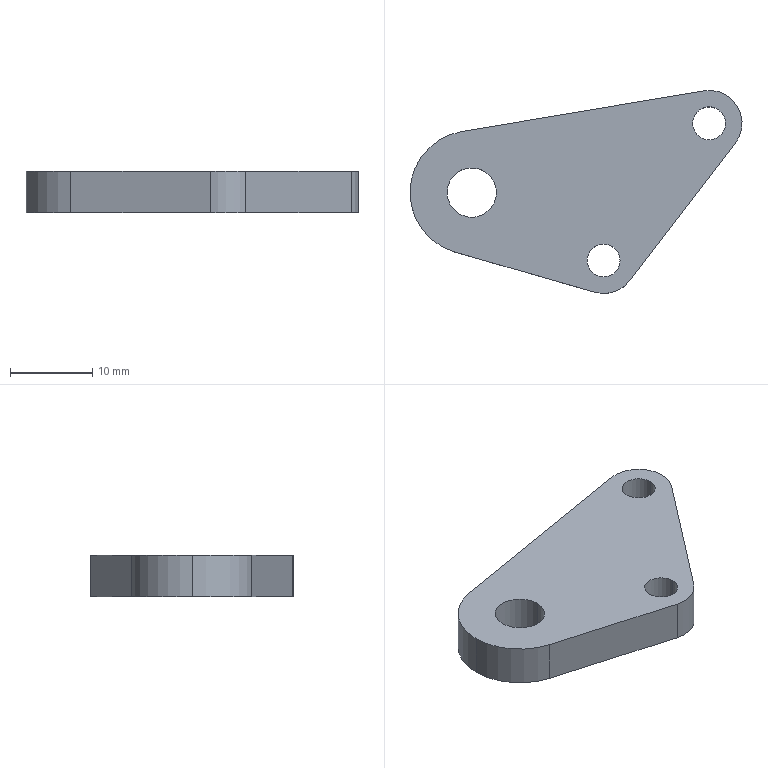Part | SolidWorks | features Extrusion 1 | 1 solid | 15 faces | box 40.3 x 24.65 x 5 mm | volume 2970 mm3 | cylinder 10 | plane 5 | commonest cylinder face diameters 4 x4 6 x2 8 x2 15 x2
STEP:
#1=CARTESIAN_POINT('',(10.8,16.65,5.));
#2=VERTEX_POINT('',#1);
#3=CARTESIAN_POINT('',(14.8,16.65,5.));
#4=VERTEX_POINT('',#3);
#5=CARTESIAN_POINT('',(12.8,16.65,5.));
#6=DIRECTION('',(0.,0.,1.));
#7=DIRECTION('',(1.,0.,0.));
#8=AXIS2_PLACEMENT_3D('',#5,#6,#7);
#9=CIRCLE('',#8,2.);
#10=EDGE_CURVE('',#2,#4,#9,.T.);
#11=ORIENTED_EDGE('',*,*,#10,.T.);
#12=CARTESIAN_POINT('',(14.8,16.65,0.));
#13=VERTEX_POINT('',#12);
#14=CARTESIAN_POINT('',(14.8,16.65,5.));
#15=DIRECTION('',(0.,0.,-1.));
#16=VECTOR('',#15,1000.);
#17=LINE('',#14,#16);
#18=EDGE_CURVE('',#4,#13,#17,.T.);
#19=ORIENTED_EDGE('',*,*,#18,.T.);
#20=CARTESIAN_POINT('',(10.8,16.65,0.));
#21=VERTEX_POINT('',#20);
#22=CARTESIAN_POINT('',(12.8,16.65,0.));
#23=DIRECTION('',(0.,0.,1.));
#24=DIRECTION('',(1.,0.,0.));
#25=AXIS2_PLACEMENT_3D('',#22,#23,#24);
#26=CIRCLE('',#25,2.);
#27=EDGE_CURVE('',#21,#13,#26,.T.);
#28=ORIENTED_EDGE('',*,*,#27,.F.);
#29=CARTESIAN_POINT('',(10.8,16.65,5.));
#30=DIRECTION('',(0.,0.,-1.));
#31=VECTOR('',#30,1000.);
#32=LINE('',#29,#31);
#33=EDGE_CURVE('',#2,#21,#32,.T.);
#34=ORIENTED_EDGE('',*,*,#33,.F.);
#35=EDGE_LOOP('',(#11,#19,#28,#34));
#36=FACE_OUTER_BOUND('',#35,.T.);
#37=CARTESIAN_POINT('',(12.8,16.65,5.));
#38=DIRECTION('',(0.,0.,-1.));
#39=DIRECTION('',(-1.,0.,0.));
#40=AXIS2_PLACEMENT_3D('',#37,#38,#39);
#41=CYLINDRICAL_SURFACE('',#40,2.);
#42=ADVANCED_FACE('',(#36),#41,.F.);
#43=CARTESIAN_POINT('',(-19.,8.25,5.));
#44=VERTEX_POINT('',#43);
#45=CARTESIAN_POINT('',(-13.,8.25,5.));
#46=VERTEX_POINT('',#45);
#47=CARTESIAN_POINT('',(-16.,8.25,5.));
#48=DIRECTION('',(0.,0.,1.));
#49=DIRECTION('',(1.,0.,0.));
#50=AXIS2_PLACEMENT_3D('',#47,#48,#49);
#51=CIRCLE('',#50,3.);
#52=EDGE_CURVE('',#44,#46,#51,.T.);
#53=ORIENTED_EDGE('',*,*,#52,.T.);
#54=CARTESIAN_POINT('',(-13.,8.25,0.));
#55=VERTEX_POINT('',#54);
#56=CARTESIAN_POINT('',(-13.,8.25,5.));
#57=DIRECTION('',(0.,0.,-1.));
#58=VECTOR('',#57,1000.);
#59=LINE('',#56,#58);
#60=EDGE_CURVE('',#46,#55,#59,.T.);
#61=ORIENTED_EDGE('',*,*,#60,.T.);
#62=CARTESIAN_POINT('',(-19.,8.25,0.));
#63=VERTEX_POINT('',#62);
#64=CARTESIAN_POINT('',(-16.,8.25,0.));
#65=DIRECTION('',(0.,0.,1.));
#66=DIRECTION('',(1.,0.,0.));
#67=AXIS2_PLACEMENT_3D('',#64,#65,#66);
#68=CIRCLE('',#67,3.);
#69=EDGE_CURVE('',#63,#55,#68,.T.);
#70=ORIENTED_EDGE('',*,*,#69,.F.);
#71=CARTESIAN_POINT('',(-19.,8.25,5.));
#72=DIRECTION('',(0.,0.,-1.));
#73=VECTOR('',#72,1000.);
#74=LINE('',#71,#73);
#75=EDGE_CURVE('',#44,#63,#74,.T.);
#76=ORIENTED_EDGE('',*,*,#75,.F.);
#77=EDGE_LOOP('',(#53,#61,#70,#76));
#78=FACE_OUTER_BOUND('',#77,.T.);
#79=CARTESIAN_POINT('',(-16.,8.25,5.));
#80=DIRECTION('',(0.,0.,-1.));
#81=DIRECTION('',(-1.,0.,0.));
#82=AXIS2_PLACEMENT_3D('',#79,#80,#81);
#83=CYLINDRICAL_SURFACE('',#82,3.);
#84=ADVANCED_FACE('',(#78),#83,.F.);
#85=CARTESIAN_POINT('',(-2.,0.,5.));
#86=VERTEX_POINT('',#85);
#87=CARTESIAN_POINT('',(2.,0.,5.));
#88=VERTEX_POINT('',#87);
#89=CARTESIAN_POINT('',(0.,0.,5.));
#90=DIRECTION('',(0.,0.,1.));
#91=DIRECTION('',(1.,0.,0.));
#92=AXIS2_PLACEMENT_3D('',#89,#90,#91);
#93=CIRCLE('',#92,2.);
#94=EDGE_CURVE('',#86,#88,#93,.T.);
#95=ORIENTED_EDGE('',*,*,#94,.T.);
#96=CARTESIAN_POINT('',(2.,0.,0.));
#97=VERTEX_POINT('',#96);
#98=CARTESIAN_POINT('',(2.,0.,5.));
#99=DIRECTION('',(0.,0.,-1.));
#100=VECTOR('',#99,1000.);
#101=LINE('',#98,#100);
#102=EDGE_CURVE('',#88,#97,#101,.T.);
#103=ORIENTED_EDGE('',*,*,#102,.T.);
#104=CARTESIAN_POINT('',(-2.,0.,0.));
#105=VERTEX_POINT('',#104);
#106=CARTESIAN_POINT('',(0.,0.,0.));
#107=DIRECTION('',(0.,0.,1.));
#108=DIRECTION('',(1.,0.,0.));
#109=AXIS2_PLACEMENT_3D('',#106,#107,#108);
#110=CIRCLE('',#109,2.);
#111=EDGE_CURVE('',#105,#97,#110,.T.);
#112=ORIENTED_EDGE('',*,*,#111,.F.);
#113=CARTESIAN_POINT('',(-2.,0.,5.));
#114=DIRECTION('',(0.,0.,-1.));
#115=VECTOR('',#114,1000.);
#116=LINE('',#113,#115);
#117=EDGE_CURVE('',#86,#105,#116,.T.);
#118=ORIENTED_EDGE('',*,*,#117,.F.);
#119=EDGE_LOOP('',(#95,#103,#112,#118));
#120=FACE_OUTER_BOUND('',#119,.T.);
#121=CARTESIAN_POINT('',(0.,0.,5.));
#122=DIRECTION('',(0.,0.,-1.));
#123=DIRECTION('',(-1.,0.,0.));
#124=AXIS2_PLACEMENT_3D('',#121,#122,#123);
#125=CYLINDRICAL_SURFACE('',#124,2.);
#126=ADVANCED_FACE('',(#120),#125,.F.);
#127=CARTESIAN_POINT('',(-23.5,8.25,5.));
#128=VERTEX_POINT('',#127);
#129=CARTESIAN_POINT('',(-18.076,1.043,5.));
#130=VERTEX_POINT('',#129);
#131=CARTESIAN_POINT('',(-16.,8.25,5.));
#132=DIRECTION('',(0.,0.,1.));
#133=DIRECTION('',(1.,0.,0.));
#134=AXIS2_PLACEMENT_3D('',#131,#132,#133);
#135=CIRCLE('',#134,7.5);
#136=EDGE_CURVE('',#128,#130,#135,.T.);
#137=ORIENTED_EDGE('',*,*,#136,.F.);
#138=CARTESIAN_POINT('',(-23.5,8.25,0.));
#139=VERTEX_POINT('',#138);
#140=CARTESIAN_POINT('',(-23.5,8.25,5.));
#141=DIRECTION('',(0.,0.,-1.));
#142=VECTOR('',#141,1000.);
#143=LINE('',#140,#142);
#144=EDGE_CURVE('',#128,#139,#143,.T.);
#145=ORIENTED_EDGE('',*,*,#144,.T.);
#146=CARTESIAN_POINT('',(-18.076,1.043,0.));
#147=VERTEX_POINT('',#146);
#148=CARTESIAN_POINT('',(-16.,8.25,0.));
#149=DIRECTION('',(0.,0.,1.));
#150=DIRECTION('',(1.,0.,0.));
#151=AXIS2_PLACEMENT_3D('',#148,#149,#150);
#152=CIRCLE('',#151,7.5);
#153=EDGE_CURVE('',#139,#147,#152,.T.);
#154=ORIENTED_EDGE('',*,*,#153,.T.);
#155=CARTESIAN_POINT('',(-18.076,1.043,5.));
#156=DIRECTION('',(0.,0.,-1.));
#157=VECTOR('',#156,1000.);
#158=LINE('',#155,#157);
#159=EDGE_CURVE('',#130,#147,#158,.T.);
#160=ORIENTED_EDGE('',*,*,#159,.F.);
#161=EDGE_LOOP('',(#137,#145,#154,#160));
#162=FACE_OUTER_BOUND('',#161,.T.);
#163=CARTESIAN_POINT('',(-16.,8.25,5.));
#164=DIRECTION('',(0.,0.,-1.));
#165=DIRECTION('',(-1.,0.,0.));
#166=AXIS2_PLACEMENT_3D('',#163,#164,#165);
#167=CYLINDRICAL_SURFACE('',#166,7.5);
#168=ADVANCED_FACE('',(#162),#167,.T.);
#169=ORIENTED_EDGE('',*,*,#52,.F.);
#170=CARTESIAN_POINT('',(-16.,8.25,5.));
#171=DIRECTION('',(0.,0.,1.));
#172=DIRECTION('',(1.,0.,0.));
#173=AXIS2_PLACEMENT_3D('',#170,#171,#172);
#174=CIRCLE('',#173,3.);
#175=EDGE_CURVE('',#46,#44,#174,.T.);
#176=ORIENTED_EDGE('',*,*,#175,.F.);
#177=EDGE_LOOP('',(#169,#176));
#178=FACE_BOUND('',#177,.T.);
#179=CARTESIAN_POINT('',(-17.246,15.646,5.));
#180=VERTEX_POINT('',#179);
#181=CARTESIAN_POINT('',(-16.,8.25,5.));
#182=DIRECTION('',(0.,0.,1.));
#183=DIRECTION('',(1.,0.,0.));
#184=AXIS2_PLACEMENT_3D('',#181,#182,#183);
#185=CIRCLE('',#184,7.5);
#186=EDGE_CURVE('',#180,#128,#185,.T.);
#187=ORIENTED_EDGE('',*,*,#186,.T.);
#188=ORIENTED_EDGE('',*,*,#136,.T.);
#189=CARTESIAN_POINT('',(-1.107,-3.844,5.));
#190=VERTEX_POINT('',#189);
#191=CARTESIAN_POINT('',(-18.076,1.043,5.));
#192=DIRECTION('',(0.9609,-0.2767,0.));
#193=VECTOR('',#192,1000.);
#194=LINE('',#191,#193);
#195=EDGE_CURVE('',#130,#190,#194,.T.);
#196=ORIENTED_EDGE('',*,*,#195,.T.);
#197=CARTESIAN_POINT('',(3.171,-2.438,5.));
#198=VERTEX_POINT('',#197);
#199=CARTESIAN_POINT('',(0.,0.,5.));
#200=DIRECTION('',(0.,0.,1.));
#201=DIRECTION('',(1.,0.,0.));
#202=AXIS2_PLACEMENT_3D('',#199,#200,#201);
#203=CIRCLE('',#202,4.);
#204=EDGE_CURVE('',#190,#198,#203,.T.);
#205=ORIENTED_EDGE('',*,*,#204,.T.);
#206=CARTESIAN_POINT('',(15.971,14.212,5.));
#207=VERTEX_POINT('',#206);
#208=CARTESIAN_POINT('',(15.971,14.212,5.));
#209=DIRECTION('',(0.6095,0.7928,0.));
#210=VECTOR('',#209,1000.);
#211=LINE('',#208,#210);
#212=EDGE_CURVE('',#198,#207,#211,.T.);
#213=ORIENTED_EDGE('',*,*,#212,.T.);
#214=CARTESIAN_POINT('',(12.136,20.594,5.));
#215=VERTEX_POINT('',#214);
#216=CARTESIAN_POINT('',(12.8,16.65,5.));
#217=DIRECTION('',(0.,0.,1.));
#218=DIRECTION('',(1.,0.,0.));
#219=AXIS2_PLACEMENT_3D('',#216,#217,#218);
#220=CIRCLE('',#219,4.);
#221=EDGE_CURVE('',#207,#215,#220,.T.);
#222=ORIENTED_EDGE('',*,*,#221,.T.);
#223=CARTESIAN_POINT('',(-17.246,15.646,5.));
#224=DIRECTION('',(-0.9861,-0.1661,0.));
#225=VECTOR('',#224,1000.);
#226=LINE('',#223,#225);
#227=EDGE_CURVE('',#215,#180,#226,.T.);
#228=ORIENTED_EDGE('',*,*,#227,.T.);
#229=EDGE_LOOP('',(#187,#188,#196,#205,#213,#222,#228));
#230=FACE_OUTER_BOUND('',#229,.T.);
#231=ORIENTED_EDGE('',*,*,#94,.F.);
#232=CARTESIAN_POINT('',(0.,0.,5.));
#233=DIRECTION('',(0.,0.,1.));
#234=DIRECTION('',(1.,0.,0.));
#235=AXIS2_PLACEMENT_3D('',#232,#233,#234);
#236=CIRCLE('',#235,2.);
#237=EDGE_CURVE('',#88,#86,#236,.T.);
#238=ORIENTED_EDGE('',*,*,#237,.F.);
#239=EDGE_LOOP('',(#231,#238));
#240=FACE_BOUND('',#239,.T.);
#241=ORIENTED_EDGE('',*,*,#10,.F.);
#242=CARTESIAN_POINT('',(12.8,16.65,5.));
#243=DIRECTION('',(0.,0.,1.));
#244=DIRECTION('',(1.,0.,0.));
#245=AXIS2_PLACEMENT_3D('',#242,#243,#244);
#246=CIRCLE('',#245,2.);
#247=EDGE_CURVE('',#4,#2,#246,.T.);
#248=ORIENTED_EDGE('',*,*,#247,.F.);
#249=EDGE_LOOP('',(#241,#248));
#250=FACE_BOUND('',#249,.T.);
#251=CARTESIAN_POINT('',(-16.,8.25,5.));
#252=DIRECTION('',(0.,0.,1.));
#253=DIRECTION('',(1.,0.,0.));
#254=AXIS2_PLACEMENT_3D('',#251,#252,#253);
#255=PLANE('',#254);
#256=ADVANCED_FACE('',(#178,#230,#240,#250),#255,.T.);
#257=CARTESIAN_POINT('',(-17.246,15.646,0.));
#258=VERTEX_POINT('',#257);
#259=CARTESIAN_POINT('',(-16.,8.25,0.));
#260=DIRECTION('',(0.,0.,1.));
#261=DIRECTION('',(1.,0.,0.));
#262=AXIS2_PLACEMENT_3D('',#259,#260,#261);
#263=CIRCLE('',#262,7.5);
#264=EDGE_CURVE('',#258,#139,#263,.T.);
#265=ORIENTED_EDGE('',*,*,#264,.F.);
#266=CARTESIAN_POINT('',(12.136,20.594,0.));
#267=VERTEX_POINT('',#266);
#268=CARTESIAN_POINT('',(-17.246,15.646,0.));
#269=DIRECTION('',(-0.9861,-0.1661,0.));
#270=VECTOR('',#269,1000.);
#271=LINE('',#268,#270);
#272=EDGE_CURVE('',#267,#258,#271,.T.);
#273=ORIENTED_EDGE('',*,*,#272,.F.);
#274=CARTESIAN_POINT('',(15.971,14.212,0.));
#275=VERTEX_POINT('',#274);
#276=CARTESIAN_POINT('',(12.8,16.65,0.));
#277=DIRECTION('',(0.,0.,1.));
#278=DIRECTION('',(1.,0.,0.));
#279=AXIS2_PLACEMENT_3D('',#276,#277,#278);
#280=CIRCLE('',#279,4.);
#281=EDGE_CURVE('',#275,#267,#280,.T.);
#282=ORIENTED_EDGE('',*,*,#281,.F.);
#283=CARTESIAN_POINT('',(3.171,-2.438,0.));
#284=VERTEX_POINT('',#283);
#285=CARTESIAN_POINT('',(15.971,14.212,0.));
#286=DIRECTION('',(0.6095,0.7928,0.));
#287=VECTOR('',#286,1000.);
#288=LINE('',#285,#287);
#289=EDGE_CURVE('',#284,#275,#288,.T.);
#290=ORIENTED_EDGE('',*,*,#289,.F.);
#291=CARTESIAN_POINT('',(-1.107,-3.844,0.));
#292=VERTEX_POINT('',#291);
#293=CARTESIAN_POINT('',(0.,0.,0.));
#294=DIRECTION('',(0.,0.,1.));
#295=DIRECTION('',(1.,0.,0.));
#296=AXIS2_PLACEMENT_3D('',#293,#294,#295);
#297=CIRCLE('',#296,4.);
#298=EDGE_CURVE('',#292,#284,#297,.T.);
#299=ORIENTED_EDGE('',*,*,#298,.F.);
#300=CARTESIAN_POINT('',(-18.076,1.043,0.));
#301=DIRECTION('',(0.9609,-0.2767,0.));
#302=VECTOR('',#301,1000.);
#303=LINE('',#300,#302);
#304=EDGE_CURVE('',#147,#292,#303,.T.);
#305=ORIENTED_EDGE('',*,*,#304,.F.);
#306=ORIENTED_EDGE('',*,*,#153,.F.);
#307=EDGE_LOOP('',(#265,#273,#282,#290,#299,#305,#306));
#308=FACE_OUTER_BOUND('',#307,.T.);
#309=ORIENTED_EDGE('',*,*,#111,.T.);
#310=CARTESIAN_POINT('',(0.,0.,0.));
#311=DIRECTION('',(0.,0.,1.));
#312=DIRECTION('',(1.,0.,0.));
#313=AXIS2_PLACEMENT_3D('',#310,#311,#312);
#314=CIRCLE('',#313,2.);
#315=EDGE_CURVE('',#97,#105,#314,.T.);
#316=ORIENTED_EDGE('',*,*,#315,.T.);
#317=EDGE_LOOP('',(#309,#316));
#318=FACE_BOUND('',#317,.T.);
#319=ORIENTED_EDGE('',*,*,#69,.T.);
#320=CARTESIAN_POINT('',(-16.,8.25,0.));
#321=DIRECTION('',(0.,0.,1.));
#322=DIRECTION('',(1.,0.,0.));
#323=AXIS2_PLACEMENT_3D('',#320,#321,#322);
#324=CIRCLE('',#323,3.);
#325=EDGE_CURVE('',#55,#63,#324,.T.);
#326=ORIENTED_EDGE('',*,*,#325,.T.);
#327=EDGE_LOOP('',(#319,#326));
#328=FACE_BOUND('',#327,.T.);
#329=ORIENTED_EDGE('',*,*,#27,.T.);
#330=CARTESIAN_POINT('',(12.8,16.65,0.));
#331=DIRECTION('',(0.,0.,1.));
#332=DIRECTION('',(1.,0.,0.));
#333=AXIS2_PLACEMENT_3D('',#330,#331,#332);
#334=CIRCLE('',#333,2.);
#335=EDGE_CURVE('',#13,#21,#334,.T.);
#336=ORIENTED_EDGE('',*,*,#335,.T.);
#337=EDGE_LOOP('',(#329,#336));
#338=FACE_BOUND('',#337,.T.);
#339=CARTESIAN_POINT('',(-16.,8.25,0.));
#340=DIRECTION('',(0.,0.,1.));
#341=DIRECTION('',(1.,0.,0.));
#342=AXIS2_PLACEMENT_3D('',#339,#340,#341);
#343=PLANE('',#342);
#344=ADVANCED_FACE('',(#308,#318,#328,#338),#343,.F.);
#345=ORIENTED_EDGE('',*,*,#144,.F.);
#346=ORIENTED_EDGE('',*,*,#186,.F.);
#347=CARTESIAN_POINT('',(-17.246,15.646,5.));
#348=DIRECTION('',(0.,0.,-1.));
#349=VECTOR('',#348,1000.);
#350=LINE('',#347,#349);
#351=EDGE_CURVE('',#180,#258,#350,.T.);
#352=ORIENTED_EDGE('',*,*,#351,.T.);
#353=ORIENTED_EDGE('',*,*,#264,.T.);
#354=EDGE_LOOP('',(#345,#346,#352,#353));
#355=FACE_OUTER_BOUND('',#354,.T.);
#356=CARTESIAN_POINT('',(-16.,8.25,5.));
#357=DIRECTION('',(0.,0.,-1.));
#358=DIRECTION('',(-1.,0.,0.));
#359=AXIS2_PLACEMENT_3D('',#356,#357,#358);
#360=CYLINDRICAL_SURFACE('',#359,7.5);
#361=ADVANCED_FACE('',(#355),#360,.T.);
#362=ORIENTED_EDGE('',*,*,#304,.T.);
#363=CARTESIAN_POINT('',(-1.107,-3.844,5.));
#364=DIRECTION('',(0.,0.,-1.));
#365=VECTOR('',#364,1000.);
#366=LINE('',#363,#365);
#367=EDGE_CURVE('',#190,#292,#366,.T.);
#368=ORIENTED_EDGE('',*,*,#367,.F.);
#369=ORIENTED_EDGE('',*,*,#195,.F.);
#370=ORIENTED_EDGE('',*,*,#159,.T.);
#371=EDGE_LOOP('',(#362,#368,#369,#370));
#372=FACE_OUTER_BOUND('',#371,.T.);
#373=CARTESIAN_POINT('',(-18.076,1.043,5.));
#374=DIRECTION('',(0.2767,0.9609,0.));
#375=DIRECTION('',(-0.9609,0.2767,0.));
#376=AXIS2_PLACEMENT_3D('',#373,#374,#375);
#377=PLANE('',#376);
#378=ADVANCED_FACE('',(#372),#377,.F.);
#379=ORIENTED_EDGE('',*,*,#298,.T.);
#380=CARTESIAN_POINT('',(3.171,-2.438,5.));
#381=DIRECTION('',(0.,0.,-1.));
#382=VECTOR('',#381,1000.);
#383=LINE('',#380,#382);
#384=EDGE_CURVE('',#198,#284,#383,.T.);
#385=ORIENTED_EDGE('',*,*,#384,.F.);
#386=ORIENTED_EDGE('',*,*,#204,.F.);
#387=ORIENTED_EDGE('',*,*,#367,.T.);
#388=EDGE_LOOP('',(#379,#385,#386,#387));
#389=FACE_OUTER_BOUND('',#388,.T.);
#390=CARTESIAN_POINT('',(0.,0.,5.));
#391=DIRECTION('',(0.,0.,-1.));
#392=DIRECTION('',(-1.,0.,0.));
#393=AXIS2_PLACEMENT_3D('',#390,#391,#392);
#394=CYLINDRICAL_SURFACE('',#393,4.);
#395=ADVANCED_FACE('',(#389),#394,.T.);
#396=ORIENTED_EDGE('',*,*,#289,.T.);
#397=CARTESIAN_POINT('',(15.971,14.212,5.));
#398=DIRECTION('',(0.,0.,-1.));
#399=VECTOR('',#398,1000.);
#400=LINE('',#397,#399);
#401=EDGE_CURVE('',#207,#275,#400,.T.);
#402=ORIENTED_EDGE('',*,*,#401,.F.);
#403=ORIENTED_EDGE('',*,*,#212,.F.);
#404=ORIENTED_EDGE('',*,*,#384,.T.);
#405=EDGE_LOOP('',(#396,#402,#403,#404));
#406=FACE_OUTER_BOUND('',#405,.T.);
#407=CARTESIAN_POINT('',(15.971,14.212,5.));
#408=DIRECTION('',(-0.7928,0.6095,0.));
#409=DIRECTION('',(-0.6095,-0.7928,0.));
#410=AXIS2_PLACEMENT_3D('',#407,#408,#409);
#411=PLANE('',#410);
#412=ADVANCED_FACE('',(#406),#411,.F.);
#413=ORIENTED_EDGE('',*,*,#281,.T.);
#414=CARTESIAN_POINT('',(12.136,20.594,5.));
#415=DIRECTION('',(0.,0.,-1.));
#416=VECTOR('',#415,1000.);
#417=LINE('',#414,#416);
#418=EDGE_CURVE('',#215,#267,#417,.T.);
#419=ORIENTED_EDGE('',*,*,#418,.F.);
#420=ORIENTED_EDGE('',*,*,#221,.F.);
#421=ORIENTED_EDGE('',*,*,#401,.T.);
#422=EDGE_LOOP('',(#413,#419,#420,#421));
#423=FACE_OUTER_BOUND('',#422,.T.);
#424=CARTESIAN_POINT('',(12.8,16.65,5.));
#425=DIRECTION('',(0.,0.,-1.));
#426=DIRECTION('',(-1.,0.,0.));
#427=AXIS2_PLACEMENT_3D('',#424,#425,#426);
#428=CYLINDRICAL_SURFACE('',#427,4.);
#429=ADVANCED_FACE('',(#423),#428,.T.);
#430=ORIENTED_EDGE('',*,*,#272,.T.);
#431=ORIENTED_EDGE('',*,*,#351,.F.);
#432=ORIENTED_EDGE('',*,*,#227,.F.);
#433=ORIENTED_EDGE('',*,*,#418,.T.);
#434=EDGE_LOOP('',(#430,#431,#432,#433));
#435=FACE_OUTER_BOUND('',#434,.T.);
#436=CARTESIAN_POINT('',(-17.246,15.646,5.));
#437=DIRECTION('',(0.1661,-0.9861,0.));
#438=DIRECTION('',(0.9861,0.1661,0.));
#439=AXIS2_PLACEMENT_3D('',#436,#437,#438);
#440=PLANE('',#439);
#441=ADVANCED_FACE('',(#435),#440,.F.);
#442=ORIENTED_EDGE('',*,*,#102,.F.);
#443=ORIENTED_EDGE('',*,*,#237,.T.);
#444=ORIENTED_EDGE('',*,*,#117,.T.);
#445=ORIENTED_EDGE('',*,*,#315,.F.);
#446=EDGE_LOOP('',(#442,#443,#444,#445));
#447=FACE_OUTER_BOUND('',#446,.T.);
#448=CARTESIAN_POINT('',(0.,0.,5.));
#449=DIRECTION('',(0.,0.,-1.));
#450=DIRECTION('',(-1.,0.,0.));
#451=AXIS2_PLACEMENT_3D('',#448,#449,#450);
#452=CYLINDRICAL_SURFACE('',#451,2.);
#453=ADVANCED_FACE('',(#447),#452,.F.);
#454=ORIENTED_EDGE('',*,*,#60,.F.);
#455=ORIENTED_EDGE('',*,*,#175,.T.);
#456=ORIENTED_EDGE('',*,*,#75,.T.);
#457=ORIENTED_EDGE('',*,*,#325,.F.);
#458=EDGE_LOOP('',(#454,#455,#456,#457));
#459=FACE_OUTER_BOUND('',#458,.T.);
#460=CARTESIAN_POINT('',(-16.,8.25,5.));
#461=DIRECTION('',(0.,0.,-1.));
#462=DIRECTION('',(-1.,0.,0.));
#463=AXIS2_PLACEMENT_3D('',#460,#461,#462);
#464=CYLINDRICAL_SURFACE('',#463,3.);
#465=ADVANCED_FACE('',(#459),#464,.F.);
#466=ORIENTED_EDGE('',*,*,#18,.F.);
#467=ORIENTED_EDGE('',*,*,#247,.T.);
#468=ORIENTED_EDGE('',*,*,#33,.T.);
#469=ORIENTED_EDGE('',*,*,#335,.F.);
#470=EDGE_LOOP('',(#466,#467,#468,#469));
#471=FACE_OUTER_BOUND('',#470,.T.);
#472=CARTESIAN_POINT('',(12.8,16.65,5.));
#473=DIRECTION('',(0.,0.,-1.));
#474=DIRECTION('',(-1.,0.,0.));
#475=AXIS2_PLACEMENT_3D('',#472,#473,#474);
#476=CYLINDRICAL_SURFACE('',#475,2.);
#477=ADVANCED_FACE('',(#471),#476,.F.);
#478=CLOSED_SHELL('',(#42,#84,#126,#168,#256,#344,#361,#378,#395,#412,#429,#441,#453,#465,#477));
#479=MANIFOLD_SOLID_BREP('',#478);
#480=CARTESIAN_POINT('',(0.,0.,0.));
#481=DIRECTION('',(0.,0.,1.));
#482=DIRECTION('',(1.,0.,0.));
#483=AXIS2_PLACEMENT_3D('',#480,#481,#482);
#484=(LENGTH_UNIT()NAMED_UNIT(*)SI_UNIT(.MILLI.,.METRE.));
#485=UNCERTAINTY_MEASURE_WITH_UNIT(LENGTH_MEASURE(0.00001),#484,'','');
#486=(NAMED_UNIT(*)PLANE_ANGLE_UNIT()SI_UNIT($,.RADIAN.));
#487=(NAMED_UNIT(*)SI_UNIT($,.STERADIAN.)SOLID_ANGLE_UNIT());
#488=(GEOMETRIC_REPRESENTATION_CONTEXT(3)GLOBAL_UNCERTAINTY_ASSIGNED_CONTEXT((#485))GLOBAL_UNIT_ASSIGNED_CONTEXT((#484,#486,#487))REPRESENTATION_CONTEXT('',''));
#489=ADVANCED_BREP_SHAPE_REPRESENTATION('',(#479,#483),#488);